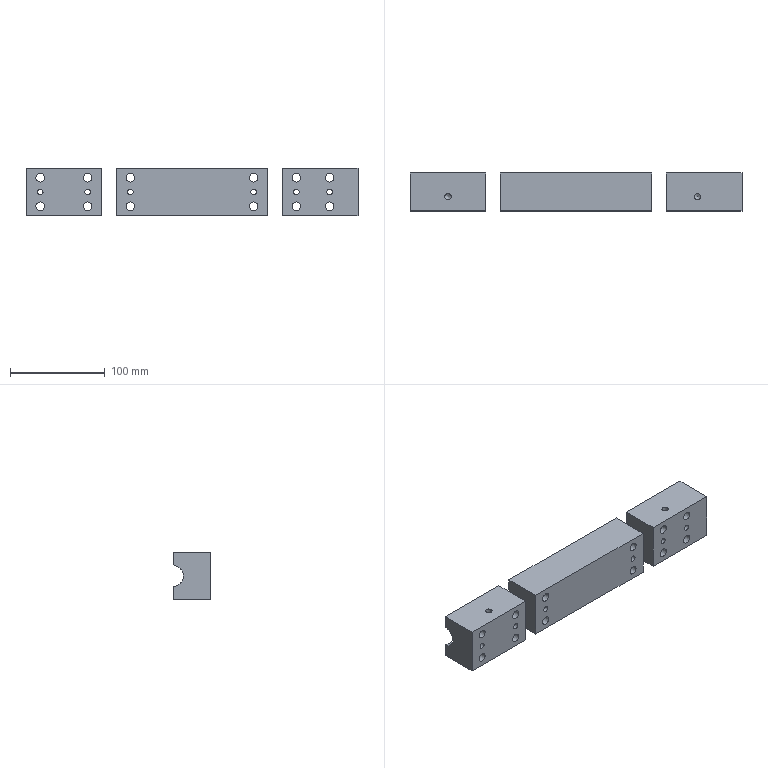Part | NX | features lower clamp 4 | 3 solids | 146 faces | box 350 x 40 x 50 mm | volume 508342 mm3 | plane 53 | spline 42 | cylinder 36 | cone 15 | commonest cylinder face diameters 9 x12 15 x12 6 x6 22.2 x3 6.8 x2 25 x1